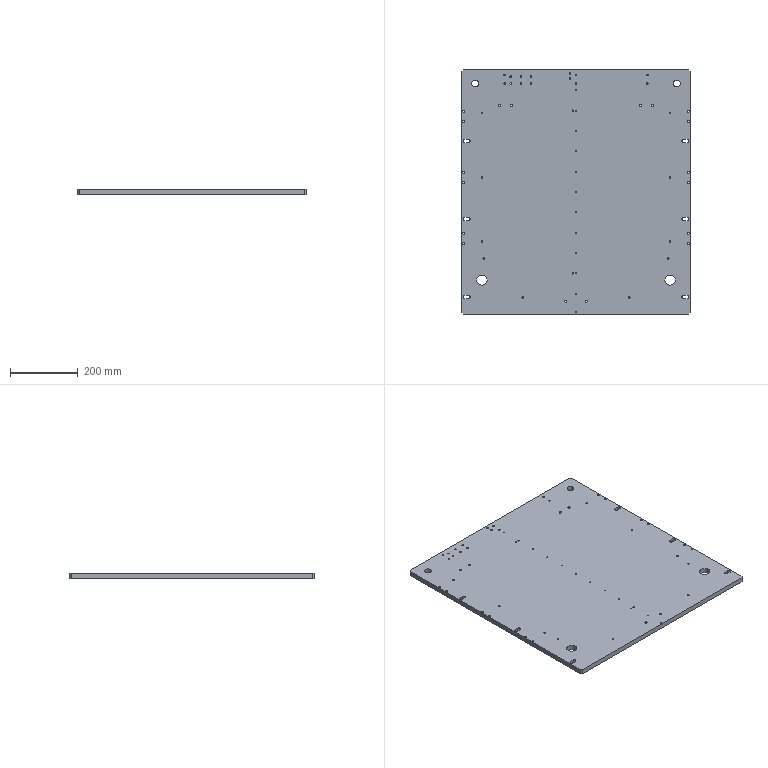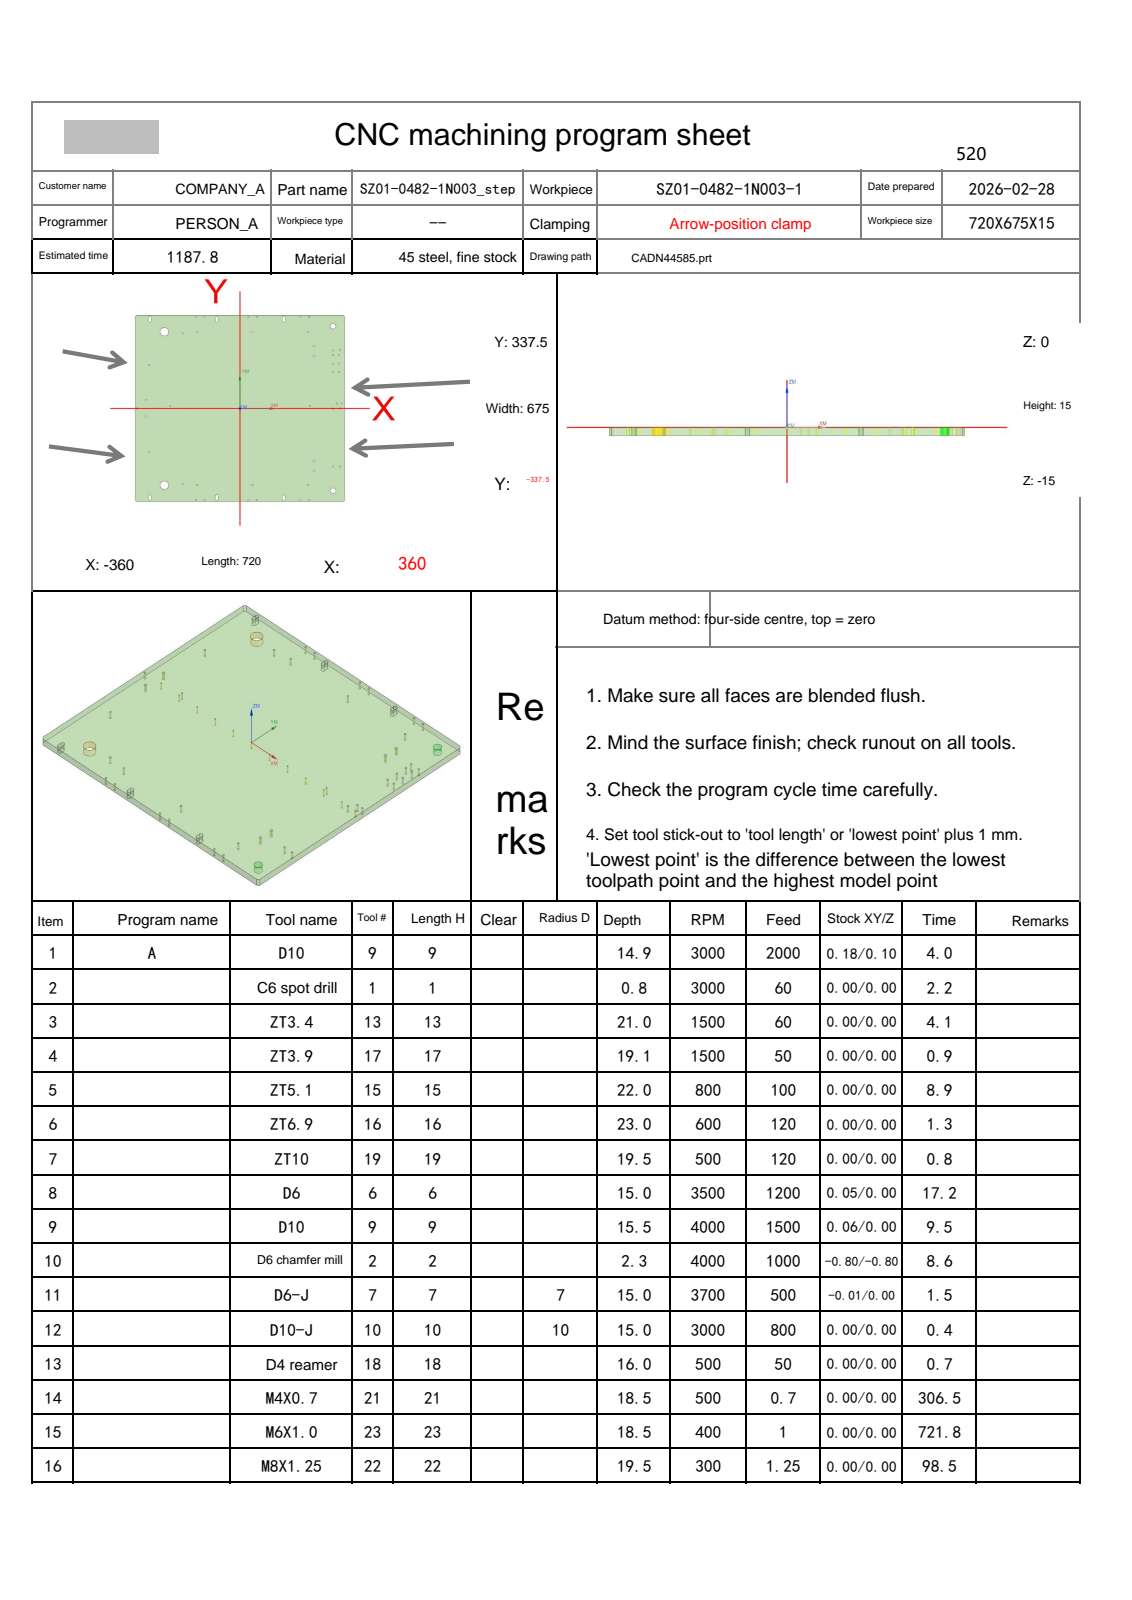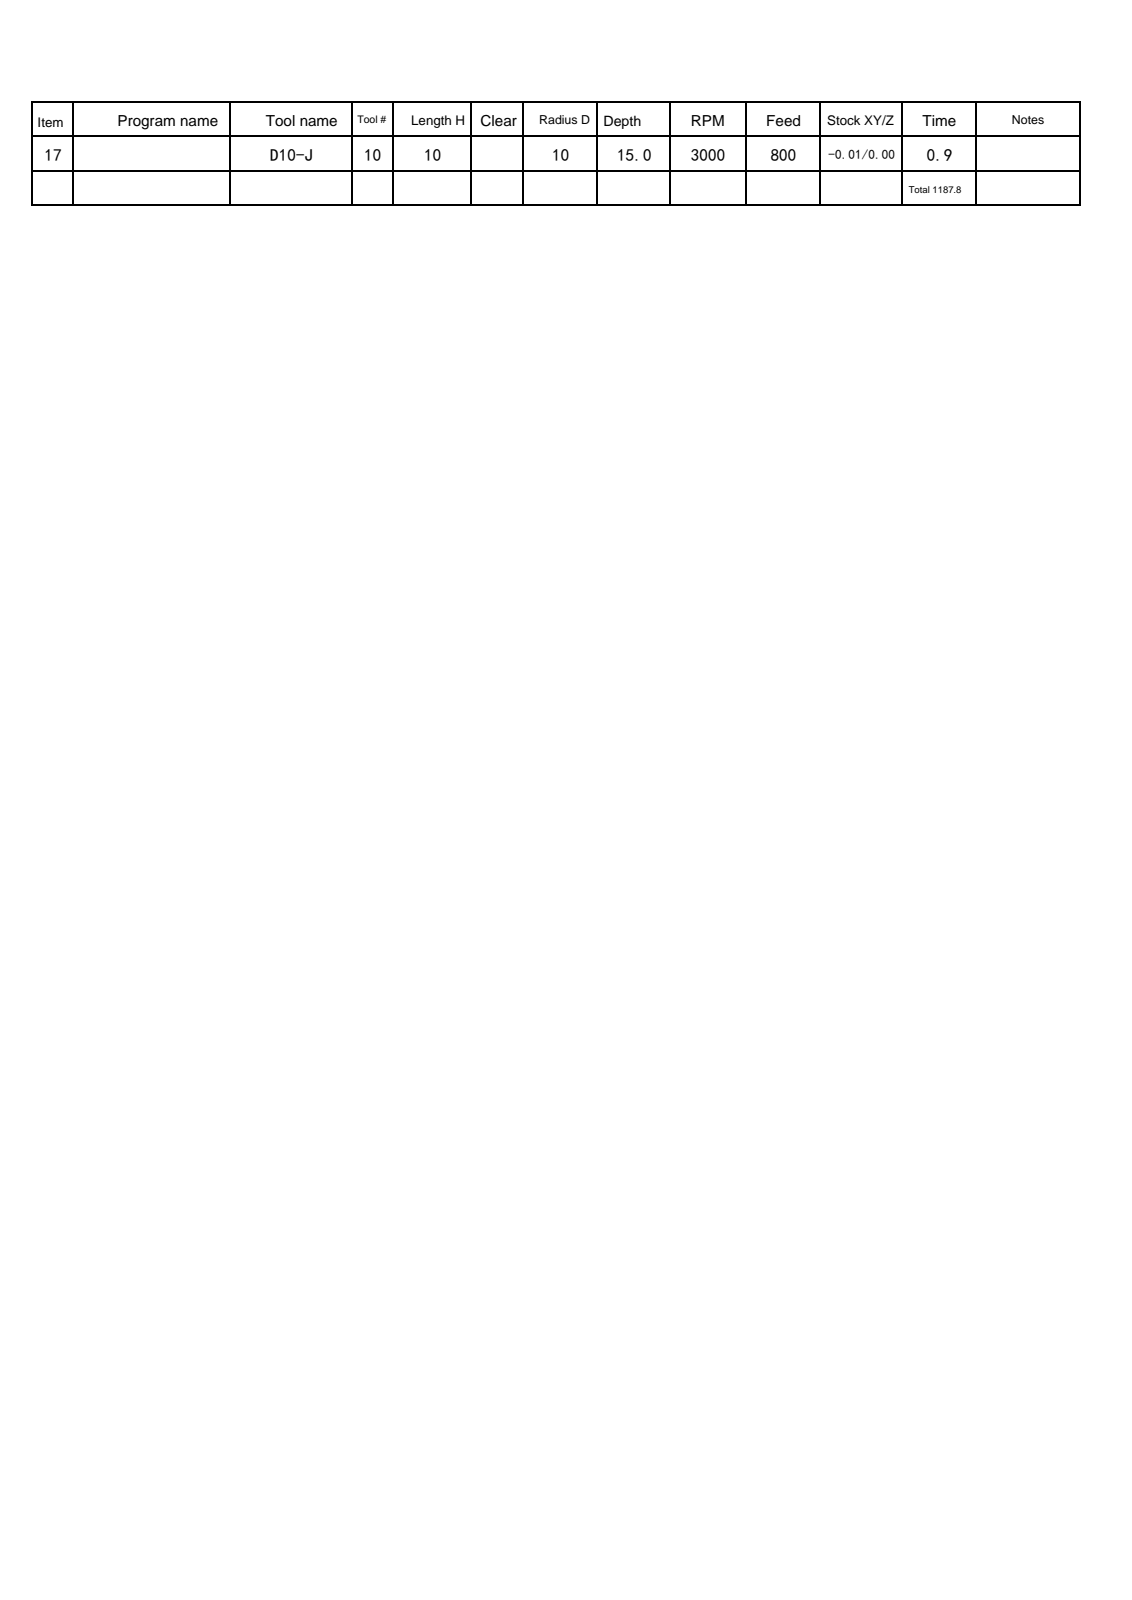NC program | NX | posted by the shop | part box 675 x 720 x 15 mm
Lines 5269 to 7670 of 7907, first 1495 of 2402 lines:
N9 T09 M06
(D10  D=10. R=0. H=09 ce=0.06 di=0.20)
G00 G90 G54 X320. Y-297.5 M03 S4000
G43 H09 Z60.
M08
Z.5
G03 X317.53 Y-299.97 I0.0 J-2.47 F1500.
X320. Y-302.44 I2.47 J0.0
X320. Y-302.44 Z.25 I0.0 J4.94
X320. Y-302.44 Z0.0 I0.0 J4.94
X320. Y-302.44 Z-.25 I0.0 J4.94
X320. Y-302.44 Z-.5 I0.0 J4.94
X320. Y-302.44 Z-.75 I0.0 J4.94
X320. Y-302.44 Z-1. I0.0 J4.94
X320. Y-302.44 Z-1.25 I0.0 J4.94
X320. Y-302.44 Z-1.5 I0.0 J4.94
X320. Y-302.44 Z-1.75 I0.0 J4.94
X320. Y-302.44 Z-2. I0.0 J4.94
X320. Y-302.44 Z-2.25 I0.0 J4.94
X320. Y-302.44 Z-2.5 I0.0 J4.94
X320. Y-302.44 Z-2.75 I0.0 J4.94
X320. Y-302.44 Z-3. I0.0 J4.94
X320. Y-302.44 Z-3.25 I0.0 J4.94
X320. Y-302.44 Z-3.5 I0.0 J4.94
X320. Y-302.44 Z-3.75 I0.0 J4.94
X320. Y-302.44 Z-4. I0.0 J4.94
X320. Y-302.44 Z-4.25 I0.0 J4.94
X320. Y-302.44 Z-4.5 I0.0 J4.94
X320. Y-302.44 Z-4.75 I0.0 J4.94
X320. Y-302.44 Z-5. I0.0 J4.94
X320. Y-302.44 Z-5.25 I0.0 J4.94
X320. Y-302.44 Z-5.5 I0.0 J4.94
X320. Y-302.44 Z-5.75 I0.0 J4.94
X320. Y-302.44 Z-6. I0.0 J4.94
X320. Y-302.44 Z-6.25 I0.0 J4.94
X320. Y-302.44 Z-6.5 I0.0 J4.94
X320. Y-302.44 Z-6.75 I0.0 J4.94
X320. Y-302.44 Z-7. I0.0 J4.94
X320. Y-302.44 Z-7.25 I0.0 J4.94
X320. Y-302.44 Z-7.5 I0.0 J4.94
X320. Y-302.44 Z-7.75 I0.0 J4.94
X320. Y-302.44 Z-8. I0.0 J4.94
X320. Y-302.44 Z-8.25 I0.0 J4.94
X320. Y-302.44 Z-8.5 I0.0 J4.94
X320. Y-302.44 Z-8.75 I0.0 J4.94
X320. Y-302.44 Z-9. I0.0 J4.94
X320. Y-302.44 Z-9.25 I0.0 J4.94
X320. Y-302.44 Z-9.5 I0.0 J4.94
X320. Y-302.44 Z-9.75 I0.0 J4.94
X320. Y-302.44 Z-10. I0.0 J4.94
X320. Y-302.44 Z-10.25 I0.0 J4.94
X320. Y-302.44 Z-10.5 I0.0 J4.94
X320. Y-302.44 Z-10.75 I0.0 J4.94
X320. Y-302.44 Z-11. I0.0 J4.94
X320. Y-302.44 Z-11.25 I0.0 J4.94
X320. Y-302.44 Z-11.5 I0.0 J4.94
X320. Y-302.44 Z-11.75 I0.0 J4.94
X320. Y-302.44 Z-12. I0.0 J4.94
X320. Y-302.44 Z-12.25 I0.0 J4.94
X320. Y-302.44 Z-12.5 I0.0 J4.94
X320. Y-302.44 Z-12.75 I0.0 J4.94
X320. Y-302.44 Z-13. I0.0 J4.94
X320. Y-302.44 Z-13.25 I0.0 J4.94
X320. Y-302.44 Z-13.5 I0.0 J4.94
X320. Y-302.44 Z-13.75 I0.0 J4.94
X320. Y-302.44 Z-14. I0.0 J4.94
X320. Y-302.44 Z-14.25 I0.0 J4.94
X320. Y-302.44 Z-14.5 I0.0 J4.94
X320. Y-302.44 Z-14.75 I0.0 J4.94
X320. Y-302.44 Z-15. I0.0 J4.94
X320. Y-302.44 Z-15.25 I0.0 J4.94
X320. Y-302.44 Z-15.5 I0.0 J4.94
X324.94 Y-297.5 I0.0 J4.94
X320. Y-292.56 I-4.94 J0.0
X315.06 Y-297.5 I0.0 J-4.94
X320. Y-302.44 I4.94 J0.0
X322.47 Y-299.97 I0.0 J2.47
X320. Y-297.5 I-2.47 J0.0
G00 Z60.
Y297.5
Z.5
G03 X317.53 Y295.03 I0.0 J-2.47
X320. Y292.56 I2.47 J0.0
X320. Y292.56 Z.25 I0.0 J4.94
X320. Y292.56 Z0.0 I0.0 J4.94
X320. Y292.56 Z-.25 I0.0 J4.94
X320. Y292.56 Z-.5 I0.0 J4.94
X320. Y292.56 Z-.75 I0.0 J4.94
X320. Y292.56 Z-1. I0.0 J4.94
X320. Y292.56 Z-1.25 I0.0 J4.94
X320. Y292.56 Z-1.5 I0.0 J4.94
X320. Y292.56 Z-1.75 I0.0 J4.94
X320. Y292.56 Z-2. I0.0 J4.94
X320. Y292.56 Z-2.25 I0.0 J4.94
X320. Y292.56 Z-2.5 I0.0 J4.94
X320. Y292.56 Z-2.75 I0.0 J4.94
X320. Y292.56 Z-3. I0.0 J4.94
X320. Y292.56 Z-3.25 I0.0 J4.94
X320. Y292.56 Z-3.5 I0.0 J4.94
X320. Y292.56 Z-3.75 I0.0 J4.94
X320. Y292.56 Z-4. I0.0 J4.94
X320. Y292.56 Z-4.25 I0.0 J4.94
X320. Y292.56 Z-4.5 I0.0 J4.94
X320. Y292.56 Z-4.75 I0.0 J4.94
X320. Y292.56 Z-5. I0.0 J4.94
X320. Y292.56 Z-5.25 I0.0 J4.94
X320. Y292.56 Z-5.5 I0.0 J4.94
X320. Y292.56 Z-5.75 I0.0 J4.94
X320. Y292.56 Z-6. I0.0 J4.94
X320. Y292.56 Z-6.25 I0.0 J4.94
X320. Y292.56 Z-6.5 I0.0 J4.94
X320. Y292.56 Z-6.75 I0.0 J4.94
X320. Y292.56 Z-7. I0.0 J4.94
X320. Y292.56 Z-7.25 I0.0 J4.94
X320. Y292.56 Z-7.5 I0.0 J4.94
X320. Y292.56 Z-7.75 I0.0 J4.94
X320. Y292.56 Z-8. I0.0 J4.94
X320. Y292.56 Z-8.25 I0.0 J4.94
X320. Y292.56 Z-8.5 I0.0 J4.94
X320. Y292.56 Z-8.75 I0.0 J4.94
X320. Y292.56 Z-9. I0.0 J4.94
X320. Y292.56 Z-9.25 I0.0 J4.94
X320. Y292.56 Z-9.5 I0.0 J4.94
X320. Y292.56 Z-9.75 I0.0 J4.94
X320. Y292.56 Z-10. I0.0 J4.94
X320. Y292.56 Z-10.25 I0.0 J4.94
X320. Y292.56 Z-10.5 I0.0 J4.94
X320. Y292.56 Z-10.75 I0.0 J4.94
X320. Y292.56 Z-11. I0.0 J4.94
X320. Y292.56 Z-11.25 I0.0 J4.94
X320. Y292.56 Z-11.5 I0.0 J4.94
X320. Y292.56 Z-11.75 I0.0 J4.94
X320. Y292.56 Z-12. I0.0 J4.94
X320. Y292.56 Z-12.25 I0.0 J4.94
X320. Y292.56 Z-12.5 I0.0 J4.94
X320. Y292.56 Z-12.75 I0.0 J4.94
X320. Y292.56 Z-13. I0.0 J4.94
X320. Y292.56 Z-13.25 I0.0 J4.94
X320. Y292.56 Z-13.5 I0.0 J4.94
X320. Y292.56 Z-13.75 I0.0 J4.94
X320. Y292.56 Z-14. I0.0 J4.94
X320. Y292.56 Z-14.25 I0.0 J4.94
X320. Y292.56 Z-14.5 I0.0 J4.94
X320. Y292.56 Z-14.75 I0.0 J4.94
X320. Y292.56 Z-15. I0.0 J4.94
X320. Y292.56 Z-15.25 I0.0 J4.94
X320. Y292.56 Z-15.5 I0.0 J4.94
X324.94 Y297.5 I0.0 J4.94
X320. Y302.44 I-4.94 J0.0
X315.06 Y297.5 I0.0 J-4.94
X320. Y292.56 I4.94 J0.0
X322.47 Y295.03 I0.0 J2.47
X320. Y297.5 I-2.47 J0.0
G00 Z60.
G00 G90 X-260. Y-277.5 M03 S4000
Z60.
Z.5
G03 X-264.97 Y-282.47 I0.0 J-4.97 F1500.
X-260. Y-287.44 I4.97 J0.0
X-260. Y-287.44 Z.3 I0.0 J9.94
X-260. Y-287.44 Z.1 I0.0 J9.94
X-260. Y-287.44 Z-.1 I0.0 J9.94
X-260. Y-287.44 Z-.3 I0.0 J9.94
X-260. Y-287.44 Z-.5 I0.0 J9.94
X-260. Y-287.44 Z-.7 I0.0 J9.94
X-260. Y-287.44 Z-.9 I0.0 J9.94
X-260. Y-287.44 Z-1.1 I0.0 J9.94
X-260. Y-287.44 Z-1.3 I0.0 J9.94
X-260. Y-287.44 Z-1.5 I0.0 J9.94
X-260. Y-287.44 Z-1.7 I0.0 J9.94
X-260. Y-287.44 Z-1.9 I0.0 J9.94
X-260. Y-287.44 Z-2.1 I0.0 J9.94
X-260. Y-287.44 Z-2.3 I0.0 J9.94
X-260. Y-287.44 Z-2.5 I0.0 J9.94
X-260. Y-287.44 Z-2.7 I0.0 J9.94
X-260. Y-287.44 Z-2.9 I0.0 J9.94
X-260. Y-287.44 Z-3.1 I0.0 J9.94
X-260. Y-287.44 Z-3.3 I0.0 J9.94
X-260. Y-287.44 Z-3.5 I0.0 J9.94
X-260. Y-287.44 Z-3.7 I0.0 J9.94
X-260. Y-287.44 Z-3.9 I0.0 J9.94
X-260. Y-287.44 Z-4.1 I0.0 J9.94
X-260. Y-287.44 Z-4.3 I0.0 J9.94
X-260. Y-287.44 Z-4.5 I0.0 J9.94
X-260. Y-287.44 Z-4.7 I0.0 J9.94
X-260. Y-287.44 Z-4.9 I0.0 J9.94
X-260. Y-287.44 Z-5.1 I0.0 J9.94
X-260. Y-287.44 Z-5.3 I0.0 J9.94
X-260. Y-287.44 Z-5.5 I0.0 J9.94
X-260. Y-287.44 Z-5.7 I0.0 J9.94
X-260. Y-287.44 Z-5.9 I0.0 J9.94
X-260. Y-287.44 Z-6.1 I0.0 J9.94
X-260. Y-287.44 Z-6.3 I0.0 J9.94
X-260. Y-287.44 Z-6.5 I0.0 J9.94
X-260. Y-287.44 Z-6.7 I0.0 J9.94
X-260. Y-287.44 Z-6.9 I0.0 J9.94
X-260. Y-287.44 Z-7.1 I0.0 J9.94
X-260. Y-287.44 Z-7.3 I0.0 J9.94
X-260. Y-287.44 Z-7.5 I0.0 J9.94
X-260. Y-287.44 Z-7.7 I0.0 J9.94
X-260. Y-287.44 Z-7.9 I0.0 J9.94
X-260. Y-287.44 Z-8.1 I0.0 J9.94
X-260. Y-287.44 Z-8.3 I0.0 J9.94
X-260. Y-287.44 Z-8.5 I0.0 J9.94
X-260. Y-287.44 Z-8.7 I0.0 J9.94
X-260. Y-287.44 Z-8.9 I0.0 J9.94
X-260. Y-287.44 Z-9.1 I0.0 J9.94
X-260. Y-287.44 Z-9.3 I0.0 J9.94
X-260. Y-287.44 Z-9.5 I0.0 J9.94
X-260. Y-287.44 Z-9.7 I0.0 J9.94
X-260. Y-287.44 Z-9.9 I0.0 J9.94
X-260. Y-287.44 Z-10.1 I0.0 J9.94
X-260. Y-287.44 Z-10.3 I0.0 J9.94
X-260. Y-287.44 Z-10.5 I0.0 J9.94
X-260. Y-287.44 Z-10.7 I0.0 J9.94
X-260. Y-287.44 Z-10.9 I0.0 J9.94
X-260. Y-287.44 Z-11.1 I0.0 J9.94
X-260. Y-287.44 Z-11.3 I0.0 J9.94
X-260. Y-287.44 Z-11.5 I0.0 J9.94
X-260. Y-287.44 Z-11.7 I0.0 J9.94
X-260. Y-287.44 Z-11.9 I0.0 J9.94
X-260. Y-287.44 Z-12.1 I0.0 J9.94
X-260. Y-287.44 Z-12.3 I0.0 J9.94
X-260. Y-287.44 Z-12.5 I0.0 J9.94
X-260. Y-287.44 Z-12.7 I0.0 J9.94
X-260. Y-287.44 Z-12.9 I0.0 J9.94
X-260. Y-287.44 Z-13.1 I0.0 J9.94
X-260. Y-287.44 Z-13.3 I0.0 J9.94
X-260. Y-287.44 Z-13.5 I0.0 J9.94
X-260. Y-287.44 Z-13.7 I0.0 J9.94
X-260. Y-287.44 Z-13.9 I0.0 J9.94
X-260. Y-287.44 Z-14.1 I0.0 J9.94
X-260. Y-287.44 Z-14.3 I0.0 J9.94
X-260. Y-287.44 Z-14.5 I0.0 J9.94
X-260. Y-287.44 Z-14.7 I0.0 J9.94
X-260. Y-287.44 Z-14.9 I0.0 J9.94
X-260. Y-267.56 Z-15. I0.0 J9.94
X-269.94 Y-277.5 I0.0 J-9.94
X-260. Y-287.44 I9.94 J0.0
X-250.06 Y-277.5 I0.0 J9.94
X-260. Y-267.56 I-9.94 J0.0
X-264.97 Y-272.53 I0.0 J-4.97
X-260. Y-277.5 I4.97 J0.0
G00 Z60.
Y277.5
Z.5
G03 X-264.97 Y272.53 I0.0 J-4.97
X-260. Y267.56 I4.97 J0.0
X-260. Y267.56 Z.3 I0.0 J9.94
X-260. Y267.56 Z.1 I0.0 J9.94
X-260. Y267.56 Z-.1 I0.0 J9.94
X-260. Y267.56 Z-.3 I0.0 J9.94
X-260. Y267.56 Z-.5 I0.0 J9.94
X-260. Y267.56 Z-.7 I0.0 J9.94
X-260. Y267.56 Z-.9 I0.0 J9.94
X-260. Y267.56 Z-1.1 I0.0 J9.94
X-260. Y267.56 Z-1.3 I0.0 J9.94
X-260. Y267.56 Z-1.5 I0.0 J9.94
X-260. Y267.56 Z-1.7 I0.0 J9.94
X-260. Y267.56 Z-1.9 I0.0 J9.94
X-260. Y267.56 Z-2.1 I0.0 J9.94
X-260. Y267.56 Z-2.3 I0.0 J9.94
X-260. Y267.56 Z-2.5 I0.0 J9.94
X-260. Y267.56 Z-2.7 I0.0 J9.94
X-260. Y267.56 Z-2.9 I0.0 J9.94
X-260. Y267.56 Z-3.1 I0.0 J9.94
X-260. Y267.56 Z-3.3 I0.0 J9.94
X-260. Y267.56 Z-3.5 I0.0 J9.94
X-260. Y267.56 Z-3.7 I0.0 J9.94
X-260. Y267.56 Z-3.9 I0.0 J9.94
X-260. Y267.56 Z-4.1 I0.0 J9.94
X-260. Y267.56 Z-4.3 I0.0 J9.94
X-260. Y267.56 Z-4.5 I0.0 J9.94
X-260. Y267.56 Z-4.7 I0.0 J9.94
X-260. Y267.56 Z-4.9 I0.0 J9.94
X-260. Y267.56 Z-5.1 I0.0 J9.94
X-260. Y267.56 Z-5.3 I0.0 J9.94
X-260. Y267.56 Z-5.5 I0.0 J9.94
X-260. Y267.56 Z-5.7 I0.0 J9.94
X-260. Y267.56 Z-5.9 I0.0 J9.94
X-260. Y267.56 Z-6.1 I0.0 J9.94
X-260. Y267.56 Z-6.3 I0.0 J9.94
X-260. Y267.56 Z-6.5 I0.0 J9.94
X-260. Y267.56 Z-6.7 I0.0 J9.94
X-260. Y267.56 Z-6.9 I0.0 J9.94
X-260. Y267.56 Z-7.1 I0.0 J9.94
X-260. Y267.56 Z-7.3 I0.0 J9.94
X-260. Y267.56 Z-7.5 I0.0 J9.94
X-260. Y267.56 Z-7.7 I0.0 J9.94
X-260. Y267.56 Z-7.9 I0.0 J9.94
X-260. Y267.56 Z-8.1 I0.0 J9.94
X-260. Y267.56 Z-8.3 I0.0 J9.94
X-260. Y267.56 Z-8.5 I0.0 J9.94
X-260. Y267.56 Z-8.7 I0.0 J9.94
X-260. Y267.56 Z-8.9 I0.0 J9.94
X-260. Y267.56 Z-9.1 I0.0 J9.94
X-260. Y267.56 Z-9.3 I0.0 J9.94
X-260. Y267.56 Z-9.5 I0.0 J9.94
X-260. Y267.56 Z-9.7 I0.0 J9.94
X-260. Y267.56 Z-9.9 I0.0 J9.94
X-260. Y267.56 Z-10.1 I0.0 J9.94
X-260. Y267.56 Z-10.3 I0.0 J9.94
X-260. Y267.56 Z-10.5 I0.0 J9.94
X-260. Y267.56 Z-10.7 I0.0 J9.94
X-260. Y267.56 Z-10.9 I0.0 J9.94
X-260. Y267.56 Z-11.1 I0.0 J9.94
X-260. Y267.56 Z-11.3 I0.0 J9.94
X-260. Y267.56 Z-11.5 I0.0 J9.94
X-260. Y267.56 Z-11.7 I0.0 J9.94
X-260. Y267.56 Z-11.9 I0.0 J9.94
X-260. Y267.56 Z-12.1 I0.0 J9.94
X-260. Y267.56 Z-12.3 I0.0 J9.94
X-260. Y267.56 Z-12.5 I0.0 J9.94
X-260. Y267.56 Z-12.7 I0.0 J9.94
X-260. Y267.56 Z-12.9 I0.0 J9.94
X-260. Y267.56 Z-13.1 I0.0 J9.94
X-260. Y267.56 Z-13.3 I0.0 J9.94
X-260. Y267.56 Z-13.5 I0.0 J9.94
X-260. Y267.56 Z-13.7 I0.0 J9.94
X-260. Y267.56 Z-13.9 I0.0 J9.94
X-260. Y267.56 Z-14.1 I0.0 J9.94
X-260. Y267.56 Z-14.3 I0.0 J9.94
X-260. Y267.56 Z-14.5 I0.0 J9.94
X-260. Y267.56 Z-14.7 I0.0 J9.94
X-260. Y267.56 Z-14.9 I0.0 J9.94
X-260. Y287.44 Z-15. I0.0 J9.94
X-269.94 Y277.5 I0.0 J-9.94
X-260. Y267.56 I9.94 J0.0
X-250.06 Y277.5 I0.0 J9.94
X-260. Y287.44 I-9.94 J0.0
X-264.97 Y282.47 I0.0 J-4.97
X-260. Y277.5 I4.97 J0.0
G00 Z60.
G91 G28 Z0.0
M05
M09
G91 G28 Z0.0
M01
N10 T02 M06
(D6 chamfer mill  D=6. R=0. H=02 ce=0.00 di=0.00)
G00 G90 G54 X-300. Y0.0 M03 S4000
G43 H02 Z30.
M08
G98 G81 X-300. Y0.0 Z-2.2 R3. F80.
X-240.
X-180.
X-120.
X-60.
X0.0
X60.
X120.
X180.
X240.
X300.
G80
G00 Z30.
G00 G90 X240. Y9.5 M03 S4000
Z30.
G98 G81 X240. Y9.5 Z-2.3 R3. F80.
X-240.
G80
G00 Z30.
G00 G90 X321.021 Y.409 M03 S4000
Z60.
Z-.6
G01 Z-1.1 F300.
X321.5 Y.6
G03 X320. Y2.1 I-1.5 J0.0
X317.9 Y0.0 I0.0 J-2.1
X320. Y-2.1 I2.1 J0.0
X322.1 Y0.0 I0.0 J2.1
X320. Y2.1 I-2.1 J0.0
X318.5 Y.6 I0.0 J-1.5
G01 X318.979 Y.409
Z-.6
G00 Z60.
X346.021
Z-.6
G01 Z-1.1
X346.5 Y.6
G03 X345. Y2.1 I-1.5 J0.0
X342.9 Y0.0 I0.0 J-2.1
X345. Y-2.1 I2.1 J0.0
X347.1 Y0.0 I0.0 J2.1
X345. Y2.1 I-2.1 J0.0
X343.5 Y.6 I0.0 J-1.5
G01 X343.979 Y.409
Z-.6
G00 Z60.
X351.021 Y18.409
Z-.6
G01 Z-1.1
X351.5 Y18.6
G03 X350. Y20.1 I-1.5 J0.0
X347.9 Y18. I0.0 J-2.1
X350. Y15.9 I2.1 J0.0
X352.1 Y18. I0.0 J2.1
X350. Y20.1 I-2.1 J0.0
X348.5 Y18.6 I0.0 J-1.5
G01 X348.979 Y18.409
Z-.6
G00 Z60.
X335.021
Z-.6
G01 Z-1.1
X335.5 Y18.6
G03 X334. Y20.1 I-1.5 J0.0
X331.9 Y18. I0.0 J-2.1
X334. Y15.9 I2.1 J0.0
X336.1 Y18. I0.0 J2.1
X334. Y20.1 I-2.1 J0.0
X332.5 Y18.6 I0.0 J-1.5
G01 X332.979 Y18.409
Z-.6
G00 Z60.
X318.979 Y132.091
Z-.6
G01 Z-1.1
X318.5 Y131.9
G03 X320. Y130.4 I1.5 J0.0
X322.1 Y132.5 I0.0 J2.1
X320. Y134.6 I-2.1 J0.0
X317.9 Y132.5 I0.0 J-2.1
X320. Y130.4 I2.1 J0.0
X321.5 Y131.9 I0.0 J1.5
G01 X321.021 Y132.091
Z-.6
G00 Z60.
X338.979
Z-.6
G01 Z-1.1
X338.5 Y131.9
G03 X340. Y130.4 I1.5 J0.0
X342.1 Y132.5 I0.0 J2.1
X340. Y134.6 I-2.1 J0.0
X337.9 Y132.5 I0.0 J-2.1
X340. Y130.4 I2.1 J0.0
X341.5 Y131.9 I0.0 J1.5
G01 X341.021 Y132.091
Z-.6
G00 Z60.
X338.979 Y162.091
Z-.6
G01 Z-1.1
X338.5 Y161.9
G03 X340. Y160.4 I1.5 J0.0
X342.1 Y162.5 I0.0 J2.1
X340. Y164.6 I-2.1 J0.0
X337.9 Y162.5 I0.0 J-2.1
X340. Y160.4 I2.1 J0.0
X341.5 Y161.9 I0.0 J1.5
G01 X341.021 Y162.091
Z-.6
G00 Z60.
X318.979
Z-.6
G01 Z-1.1
X318.5 Y161.9
G03 X320. Y160.4 I1.5 J0.0
X322.1 Y162.5 I0.0 J2.1
X320. Y164.6 I-2.1 J0.0
X317.9 Y162.5 I0.0 J-2.1
X320. Y160.4 I2.1 J0.0
X321.5 Y161.9 I0.0 J1.5
G01 X321.021 Y162.091
Z-.6
G00 Z60.
X318.979 Y192.091
Z-.6
G01 Z-1.1
X318.5 Y191.9
G03 X320. Y190.4 I1.5 J0.0
X322.1 Y192.5 I0.0 J2.1
X320. Y194.6 I-2.1 J0.0
X317.9 Y192.5 I0.0 J-2.1
X320. Y190.4 I2.1 J0.0
X321.5 Y191.9 I0.0 J1.5
G01 X321.021 Y192.091
Z-.6
G00 Z60.
X338.979
Z-.6
G01 Z-1.1
X338.5 Y191.9
G03 X340. Y190.4 I1.5 J0.0
X342.1 Y192.5 I0.0 J2.1
X340. Y194.6 I-2.1 J0.0
X337.9 Y192.5 I0.0 J-2.1
X340. Y190.4 I2.1 J0.0
X341.5 Y191.9 I0.0 J1.5
G01 X341.021 Y192.091
Z-.6
G00 Z60.
X346.021 Y210.409
Z-.6
G01 Z-1.1
X346.5 Y210.6
G03 X345. Y212.1 I-1.5 J0.0
X342.9 Y210. I0.0 J-2.1
X345. Y207.9 I2.1 J0.0
X347.1 Y210. I0.0 J2.1
X345. Y212.1 I-2.1 J0.0
X343.5 Y210.6 I0.0 J-1.5
G01 X343.979 Y210.409
Z-.6
G00 Z60.
X321.021
Z-.6
G01 Z-1.1
X321.5 Y210.6
G03 X320. Y212.1 I-1.5 J0.0
X317.9 Y210. I0.0 J-2.1
X320. Y207.9 I2.1 J0.0
X322.1 Y210. I0.0 J2.1
X320. Y212.1 I-2.1 J0.0
X318.5 Y210.6 I0.0 J-1.5
G01 X318.979 Y210.409
Z-.6
G00 Z60.
X234.021 Y277.409
Z-.6
G01 Z-1.1
X234.5 Y277.6
G03 X233. Y279.1 I-1.5 J0.0
X230.9 Y277. I0.0 J-2.1
X233. Y274.9 I2.1 J0.0
X235.1 Y277. I0.0 J2.1
X233. Y279.1 I-2.1 J0.0
X231.5 Y277.6 I0.0 J-1.5
G01 X231.979 Y277.409
Z-.6
G00 Z60.
X239.021 Y331.909
Z-.6
G01 Z-1.1
X239.5 Y332.1
G03 X238. Y333.6 I-1.5 J0.0
X235.9 Y331.5 I0.0 J-2.1
X238. Y329.4 I2.1 J0.0
X240.1 Y331.5 I0.0 J2.1
X238. Y333.6 I-2.1 J0.0
X236.5 Y332.1 I0.0 J-1.5
G01 X236.979 Y331.909
Z-.6
G00 Z60.
X209.021
Z-.6
G01 Z-1.1
X209.5 Y332.1
G03 X208. Y333.6 I-1.5 J0.0
X205.9 Y331.5 I0.0 J-2.1
X208. Y329.4 I2.1 J0.0
X210.1 Y331.5 I0.0 J2.1
X208. Y333.6 I-2.1 J0.0
X206.5 Y332.1 I0.0 J-1.5
G01 X206.979 Y331.909
Z-.6
G00 Z60.
X59.021
Z-.6
G01 Z-1.1
X59.5 Y332.1
G03 X58. Y333.6 I-1.5 J0.0
X55.9 Y331.5 I0.0 J-2.1
X58. Y329.4 I2.1 J0.0
X60.1 Y331.5 I0.0 J2.1
X58. Y333.6 I-2.1 J0.0
X56.5 Y332.1 I0.0 J-1.5
G01 X56.979 Y331.909
Z-.6
G00 Z60.
X44.021 Y277.409
Z-.6
G01 Z-1.1
X44.5 Y277.6
G03 X43. Y279.1 I-1.5 J0.0
X40.9 Y277. I0.0 J-2.1
X43. Y274.9 I2.1 J0.0
X45.1 Y277. I0.0 J2.1
X43. Y279.1 I-2.1 J0.0
X41.5 Y277.6 I0.0 J-1.5
G01 X41.979 Y277.409
Z-.6
G00 Z60.
X29.021 Y331.909
Z-.6
G01 Z-1.1
X29.5 Y332.1
G03 X28. Y333.6 I-1.5 J0.0
X25.9 Y331.5 I0.0 J-2.1
X28. Y329.4 I2.1 J0.0
X30.1 Y331.5 I0.0 J2.1
X28. Y333.6 I-2.1 J0.0
X26.5 Y332.1 I0.0 J-1.5
G01 X26.979 Y331.909
Z-.6
G00 Z60.
X-120.979
Z-.6
G01 Z-1.1
X-120.5 Y332.1
G03 X-122. Y333.6 I-1.5 J0.0
X-124.1 Y331.5 I0.0 J-2.1
X-122. Y329.4 I2.1 J0.0
X-119.9 Y331.5 I0.0 J2.1
X-122. Y333.6 I-2.1 J0.0
X-123.5 Y332.1 I0.0 J-1.5
G01 X-123.021 Y331.909
Z-.6
G00 Z60.
X-150.979
Z-.6
G01 Z-1.1
X-150.5 Y332.1
G03 X-152. Y333.6 I-1.5 J0.0
X-154.1 Y331.5 I0.0 J-2.1
X-152. Y329.4 I2.1 J0.0
X-149.9 Y331.5 I0.0 J2.1
X-152. Y333.6 I-2.1 J0.0
X-153.5 Y332.1 I0.0 J-1.5
G01 X-153.021 Y331.909
Z-.6
G00 Z60.
X-145.979 Y277.409
Z-.6
G01 Z-1.1
X-145.5 Y277.6
G03 X-147. Y279.1 I-1.5 J0.0
X-149.1 Y277. I0.0 J-2.1
X-147. Y274.9 I2.1 J0.0
X-144.9 Y277. I0.0 J2.1
X-147. Y279.1 I-2.1 J0.0
X-148.5 Y277.6 I0.0 J-1.5
G01 X-148.021 Y277.409
Z-.6
G00 Z60.
X-195.979 Y272.341
Z-.6
G01 Z-1.1
X-195.5 Y272.532
G03 X-197. Y274.032 I-1.5 J0.0
X-199.1 Y271.932 I0.0 J-2.1
X-197. Y269.832 I2.1 J0.0
X-194.9 Y271.932 I0.0 J2.1
X-197. Y274.032 I-2.1 J0.0
X-198.5 Y272.532 I0.0 J-1.5
G01 X-198.021 Y272.341
Z-.6
G00 Z60.
X-310.911 Y157.409
Z-.6
G01 Z-1.1
X-310.432 Y157.6
G03 X-311.932 Y159.1 I-1.5 J0.0
X-314.032 Y157. I0.0 J-2.1
X-311.932 Y154.9 I2.1 J0.0
X-309.832 Y157. I0.0 J2.1
X-311.932 Y159.1 I-2.1 J0.0
X-313.432 Y157.6 I0.0 J-1.5
G01 X-312.953 Y157.409
Z-.6
G00 Z60.
X-352.979 Y.409
Z-.6
G01 Z-1.1
X-352.5 Y.6
G03 X-354. Y2.1 I-1.5 J0.0
X-356.1 Y0.0 I0.0 J-2.1
X-354. Y-2.1 I2.1 J0.0
X-351.9 Y0.0 I0.0 J2.1
X-354. Y2.1 I-2.1 J0.0
X-355.5 Y.6 I0.0 J-1.5
G01 X-355.021 Y.409
Z-.6
G00 Z60.
X-310.911 Y-156.591
Z-.6
G01 Z-1.1
X-310.432 Y-156.4
G03 X-311.932 Y-154.9 I-1.5 J0.0
X-314.032 Y-157. I0.0 J-2.1
X-311.932 Y-159.1 I2.1 J0.0
X-309.832 Y-157. I0.0 J2.1
X-311.932 Y-154.9 I-2.1 J0.0
X-313.432 Y-156.4 I0.0 J-1.5
G01 X-312.953 Y-156.591
Z-.6
G00 Z60.
X-195.979 Y-271.523
Z-.6
G01 Z-1.1
X-195.5 Y-271.332
G03 X-197. Y-269.832 I-1.5 J0.0
X-199.1 Y-271.932 I0.0 J-2.1
X-197. Y-274.032 I2.1 J0.0
X-194.9 Y-271.932 I0.0 J2.1
X-197. Y-269.832 I-2.1 J0.0
X-198.5 Y-271.332 I0.0 J-1.5
G01 X-198.021 Y-271.523
Z-.6
G00 Z60.
X-145.979 Y-276.591
Z-.6
G01 Z-1.1
X-145.5 Y-276.4
G03 X-147. Y-274.9 I-1.5 J0.0
X-149.1 Y-277. I0.0 J-2.1
X-147. Y-279.1 I2.1 J0.0
X-144.9 Y-277. I0.0 J2.1
X-147. Y-274.9 I-2.1 J0.0
X-148.5 Y-276.4 I0.0 J-1.5
G01 X-148.021 Y-276.591
Z-.6
G00 Z60.
X-150.979 Y-331.091
Z-.6
G01 Z-1.1
X-150.5 Y-330.9
G03 X-152. Y-329.4 I-1.5 J0.0
X-154.1 Y-331.5 I0.0 J-2.1
X-152. Y-333.6 I2.1 J0.0
X-149.9 Y-331.5 I0.0 J2.1
X-152. Y-329.4 I-2.1 J0.0
X-153.5 Y-330.9 I0.0 J-1.5
G01 X-153.021 Y-331.091
Z-.6
G00 Z60.
X-120.979
Z-.6
G01 Z-1.1
X-120.5 Y-330.9
G03 X-122. Y-329.4 I-1.5 J0.0
X-124.1 Y-331.5 I0.0 J-2.1
X-122. Y-333.6 I2.1 J0.0
X-119.9 Y-331.5 I0.0 J2.1
X-122. Y-329.4 I-2.1 J0.0
X-123.5 Y-330.9 I0.0 J-1.5
G01 X-123.021 Y-331.091
Z-.6
G00 Z60.
X29.021
Z-.6
G01 Z-1.1
X29.5 Y-330.9
G03 X28. Y-329.4 I-1.5 J0.0
X25.9 Y-331.5 I0.0 J-2.1
X28. Y-333.6 I2.1 J0.0
X30.1 Y-331.5 I0.0 J2.1
X28. Y-329.4 I-2.1 J0.0
X26.5 Y-330.9 I0.0 J-1.5
G01 X26.979 Y-331.091
Z-.6
G00 Z60.
X44.021 Y-276.591
Z-.6
G01 Z-1.1
X44.5 Y-276.4
G03 X43. Y-274.9 I-1.5 J0.0
X40.9 Y-277. I0.0 J-2.1
X43. Y-279.1 I2.1 J0.0
X45.1 Y-277. I0.0 J2.1
X43. Y-274.9 I-2.1 J0.0
X41.5 Y-276.4 I0.0 J-1.5
G01 X41.979 Y-276.591
Z-.6
G00 Z60.
X59.021 Y-331.091
Z-.6
G01 Z-1.1
X59.5 Y-330.9
G03 X58. Y-329.4 I-1.5 J0.0
X55.9 Y-331.5 I0.0 J-2.1
X58. Y-333.6 I2.1 J0.0
X60.1 Y-331.5 I0.0 J2.1
X58. Y-329.4 I-2.1 J0.0
X56.5 Y-330.9 I0.0 J-1.5
G01 X56.979 Y-331.091
Z-.6
G00 Z60.
X209.021
Z-.6
G01 Z-1.1
X209.5 Y-330.9
G03 X208. Y-329.4 I-1.5 J0.0
X205.9 Y-331.5 I0.0 J-2.1
X208. Y-333.6 I2.1 J0.0
X210.1 Y-331.5 I0.0 J2.1
X208. Y-329.4 I-2.1 J0.0
X206.5 Y-330.9 I0.0 J-1.5
G01 X206.979 Y-331.091
Z-.6
G00 Z60.
X239.021
Z-.6
G01 Z-1.1
X239.5 Y-330.9
G03 X238. Y-329.4 I-1.5 J0.0
X235.9 Y-331.5 I0.0 J-2.1
X238. Y-333.6 I2.1 J0.0
X240.1 Y-331.5 I0.0 J2.1
X238. Y-329.4 I-2.1 J0.0
X236.5 Y-330.9 I0.0 J-1.5
G01 X236.979 Y-331.091
Z-.6
G00 Z60.
X234.021 Y-276.591
Z-.6
G01 Z-1.1
X234.5 Y-276.4
G03 X233. Y-274.9 I-1.5 J0.0
X230.9 Y-277. I0.0 J-2.1
X233. Y-279.1 I2.1 J0.0
X235.1 Y-277. I0.0 J2.1
X233. Y-274.9 I-2.1 J0.0
X231.5 Y-276.4 I0.0 J-1.5
G01 X231.979 Y-276.591
Z-.6
G00 Z60.
X321.021 Y-209.591
Z-.6
G01 Z-1.1
X321.5 Y-209.4
G03 X320. Y-207.9 I-1.5 J0.0
X317.9 Y-210. I0.0 J-2.1
X320. Y-212.1 I2.1 J0.0
X322.1 Y-210. I0.0 J2.1
X320. Y-207.9 I-2.1 J0.0
X318.5 Y-209.4 I0.0 J-1.5
G01 X318.979 Y-209.591
Z-.6
G00 Z60.
X346.021
Z-.6
G01 Z-1.1
X346.5 Y-209.4
G03 X345. Y-207.9 I-1.5 J0.0
X342.9 Y-210. I0.0 J-2.1
X345. Y-212.1 I2.1 J0.0
X347.1 Y-210. I0.0 J2.1
X345. Y-207.9 I-2.1 J0.0
X343.5 Y-209.4 I0.0 J-1.5
G01 X343.979 Y-209.591
Z-.6
G00 Z60.
G00 G90 X-320.5 Y30.8 M03 S4000
Z60.
Z-1.
G01 Z-1.5 F500.
Y31.2
G03 X-322. Y32.7 I-1.5 J0.0
X-324.7 Y30. I0.0 J-2.7
X-322. Y27.3 I2.7 J0.0
X-319.3 Y30. I0.0 J2.7
X-322. Y32.7 I-2.7 J0.0
X-323.5 Y31.2 I0.0 J-1.5
G01 Y30.8
Z-1.
G00 Z60.
X-320.5 Y-29.2
Z-1.
G01 Z-1.5
Y-28.8
G03 X-322. Y-27.3 I-1.5 J0.0
X-324.7 Y-30. I0.0 J-2.7
X-322. Y-32.7 I2.7 J0.0
X-319.3 Y-30. I0.0 J2.7
X-322. Y-27.3 I-2.7 J0.0
X-323.5 Y-28.8 I0.0 J-1.5
G01 Y-29.2
Z-1.
G00 Z60.
X256.5 Y-224.7
Z-1.
G01 Z-1.5
Y-224.3
G03 X255. Y-222.8 I-1.5 J0.0
X252.3 Y-225.5 I0.0 J-2.7
X255. Y-228.2 I2.7 J0.0
X257.7 Y-225.5 I0.0 J2.7
X255. Y-222.8 I-2.7 J0.0
X253.5 Y-224.3 I0.0 J-1.5
G01 Y-224.7
Z-1.
G00 Z60.
X256.5 Y-188.7
Z-1.
G01 Z-1.5
Y-188.3
G03 X255. Y-186.8 I-1.5 J0.0
X252.3 Y-189.5 I0.0 J-2.7
X255. Y-192.2 I2.7 J0.0
X257.7 Y-189.5 I0.0 J2.7
X255. Y-186.8 I-2.7 J0.0
X253.5 Y-188.3 I0.0 J-1.5
G01 Y-188.7
Z-1.
G00 Z60.
X256.5 Y190.3
Z-1.
G01 Z-1.5
Y190.7
G03 X255. Y192.2 I-1.5 J0.0
X252.3 Y189.5 I0.0 J-2.7
X255. Y186.8 I2.7 J0.0
X257.7 Y189.5 I0.0 J2.7
X255. Y192.2 I-2.7 J0.0
X253.5 Y190.7 I0.0 J-1.5
G01 Y190.3
Z-1.
G00 Z60.
X256.5 Y226.3
Z-1.
G01 Z-1.5
Y226.7
G03 X255. Y228.2 I-1.5 J0.0
X252.3 Y225.5 I0.0 J-2.7
X255. Y222.8 I2.7 J0.0
X257.7 Y225.5 I0.0 J2.7
X255. Y228.2 I-2.7 J0.0
X253.5 Y226.7 I0.0 J-1.5
G01 Y226.3
Z-1.
G00 Z60.
G00 G90 X-361.375 Y332.257 M03 S3500
Z60.
Z.055
G01 Z-1.2 F1000.
G03 X-361.069 Y332.423 I-.795 J1.835
G01 X-361.022 Y332.45
X-361. Y332.5
X-360.966 Y332.759
X-360.866 Y333.
X-360.707 Y333.207
X-355.707 Y338.207
X-355.5 Y338.366
X-355.259 Y338.466
X-355. Y338.5
X355.
X355.259 Y338.466
X355.5 Y338.366
X355.707 Y338.207
X360.707 Y333.207
X360.744 Y333.167
X360.797 Y333.155
G03 X361.14 Y333.095 I.518 J1.932
G01 Z.113
G00 Z60.
Y-333.095
Z.113
G01 Z-1.2
G03 X360.797 Y-333.155 I.174 J-1.992
G01 X360.744 Y-333.167
X360.707 Y-333.207
X355.707 Y-338.207
X355.5 Y-338.366
X355.259 Y-338.466
X355. Y-338.5
X-355.
X-355.259 Y-338.466
X-355.5 Y-338.366
X-355.707 Y-338.207
X-360.707 Y-333.207
X-360.744 Y-333.167
X-360.797 Y-333.155
G03 X-361.14 Y-333.095 I-.518 J-1.932
G01 Z.113
G00 Z60.
X-313.773 Y-322.114
Z.172
G01 Z-1.2
G03 X-313.973 Y-322.4 I1.532 J-1.286
G01 X-314.003 Y-322.446
X-314. Y-322.5
Y-327.5
G03 X-310. Y-331.5 I4. J0.0
X-306. Y-327.5 I0.0 J4.
G01 Y-317.5
G03 X-310. Y-313.5 I-4. J0.0
X-314. Y-317.5 I0.0 J-4.
G01 Y-322.5
X-314.003 Y-322.554
X-313.973 Y-322.6
G03 X-313.773 Y-322.886 I1.732 J1.
G01 Z.172
G00 Z60.
X-311.525 Y-155.685
Z.284
G01 Z-1.2
G03 X-311.83 Y-155.516 I-1.118 J-1.658
G01 X-311.878 Y-155.491
X-311.932 Y-155.5
G03 X-313.432 Y-157. I0.0 J-1.5
X-311.932 Y-158.5 I1.5 J0.0
X-310.432 Y-157. I0.0 J1.5
X-311.932 Y-155.5 I-1.5 J0.0
G01 X-311.986 Y-155.491
X-312.034 Y-155.516
G03 X-312.339 Y-155.685 I.813 J-1.827
G01 Z.284
G00 Z60.
X-259.606 Y-263.712
Z.196
G01 Z-1.2
G03 X-259.899 Y-263.523 I-1.227 J-1.579
G01 X-259.946 Y-263.495
X-260. Y-263.5
G03 X-274. Y-277.5 I0.0 J-14.
X-260. Y-291.5 I14. J0.0
X-246. Y-277.5 I0.0 J14.
X-260. Y-263.5 I-14. J0.0
G01 X-260.054 Y-263.495
X-260.101 Y-263.523
G03 X-260.394 Y-263.712 I.935 J-1.768
G01 Z.196
G00 Z60.
X-196.593 Y-270.617
Z.284
G01 Z-1.2
G03 X-196.898 Y-270.448 I-1.118 J-1.658
G01 X-196.946 Y-270.423
X-197. Y-270.432
G03 X-198.5 Y-271.932 I0.0 J-1.5
X-197. Y-273.432 I1.5 J0.0
X-195.5 Y-271.932 I0.0 J1.5
X-197. Y-270.432 I-1.5 J0.0
G01 X-197.054 Y-270.423
X-197.102 Y-270.448
G03 X-197.407 Y-270.617 I.813 J-1.827
G01 Z.284
G00 Z60.
X-146.593 Y-275.685
Z.284
G01 Z-1.2
G03 X-146.898 Y-275.516 I-1.118 J-1.658
G01 X-146.946 Y-275.491
X-147. Y-275.5
G03 X-148.5 Y-277. I0.0 J-1.5
X-147. Y-278.5 I1.5 J0.0
X-145.5 Y-277. I0.0 J1.5
X-147. Y-275.5 I-1.5 J0.0
G01 X-147.054 Y-275.491
X-147.102 Y-275.516
G03 X-147.407 Y-275.685 I.813 J-1.827
G01 Z.284
G00 Z60.
X-151.593 Y-330.185
Z.284
G01 Z-1.2
G03 X-151.898 Y-330.016 I-1.118 J-1.658
G01 X-151.946 Y-329.991
X-152. Y-330.
G03 X-153.5 Y-331.5 I0.0 J-1.5
X-152. Y-333. I1.5 J0.0
X-150.5 Y-331.5 I0.0 J1.5
X-152. Y-330. I-1.5 J0.0
G01 X-152.054 Y-329.991
X-152.102 Y-330.016
G03 X-152.407 Y-330.185 I.813 J-1.827
G01 Z.284
G00 Z60.
X-121.593
Z.284
G01 Z-1.2
G03 X-121.898 Y-330.016 I-1.118 J-1.658
G01 X-121.946 Y-329.991
X-122. Y-330.
G03 X-123.5 Y-331.5 I0.0 J-1.5
X-122. Y-333. I1.5 J0.0
X-120.5 Y-331.5 I0.0 J1.5
X-122. Y-330. I-1.5 J0.0
G01 X-122.054 Y-329.991
X-122.102 Y-330.016
G03 X-122.407 Y-330.185 I.813 J-1.827
G01 Z.284
G00 Z60.
X-83.773 Y-322.114
Z.172
G01 Z-1.2
G03 X-83.973 Y-322.4 I1.532 J-1.286
G01 X-84.003 Y-322.446
X-84. Y-322.5
Y-327.5
G03 X-80. Y-331.5 I4. J0.0
X-76. Y-327.5 I0.0 J4.
G01 Y-317.5
G03 X-80. Y-313.5 I-4. J0.0
X-84. Y-317.5 I0.0 J-4.
G01 Y-322.5
X-84.003 Y-322.554
X-83.973 Y-322.6
G03 X-83.773 Y-322.886 I1.732 J1.
G01 Z.172
G00 Z60.
X43.407 Y-275.685
Z.284
G01 Z-1.2
G03 X43.102 Y-275.516 I-1.118 J-1.658
G01 X43.054 Y-275.491
X43. Y-275.5
G03 X41.5 Y-277. I0.0 J-1.5
X43. Y-278.5 I1.5 J0.0
X44.5 Y-277. I0.0 J1.5
X43. Y-275.5 I-1.5 J0.0
G01 X42.946 Y-275.491
X42.898 Y-275.516
G03 X42.593 Y-275.685 I.813 J-1.827
G01 Z.284
G00 Z60.
X28.407 Y-330.185
Z.284
G01 Z-1.2
G03 X28.102 Y-330.016 I-1.118 J-1.658
G01 X28.054 Y-329.991
X28. Y-330.
G03 X26.5 Y-331.5 I0.0 J-1.5
X28. Y-333. I1.5 J0.0
X29.5 Y-331.5 I0.0 J1.5
X28. Y-330. I-1.5 J0.0
G01 X27.946 Y-329.991
X27.898 Y-330.016
G03 X27.593 Y-330.185 I.813 J-1.827
G01 Z.284
G00 Z60.
X58.407
Z.284
G01 Z-1.2
G03 X58.102 Y-330.016 I-1.118 J-1.658
G01 X58.054 Y-329.991
X58. Y-330.
G03 X56.5 Y-331.5 I0.0 J-1.5
X58. Y-333. I1.5 J0.0
X59.5 Y-331.5 I0.0 J1.5
X58. Y-330. I-1.5 J0.0
G01 X57.946 Y-329.991
X57.898 Y-330.016
G03 X57.593 Y-330.185 I.813 J-1.827
G01 Z.284
G00 Z60.
X146.227 Y-322.114
Z.172
G01 Z-1.2
G03 X146.027 Y-322.4 I1.532 J-1.286
G01 X145.997 Y-322.446
X146. Y-322.5
Y-327.5
G03 X150. Y-331.5 I4. J0.0
X154. Y-327.5 I0.0 J4.
G01 Y-317.5
G03 X150. Y-313.5 I-4. J0.0
X146. Y-317.5 I0.0 J-4.
G01 Y-322.5
X145.997 Y-322.554
X146.027 Y-322.6
G03 X146.227 Y-322.886 I1.732 J1.
G01 Z.172
G00 Z60.
X208.407 Y-330.185
Z.284
G01 Z-1.2
G03 X208.102 Y-330.016 I-1.118 J-1.658
G01 X208.054 Y-329.991
X208. Y-330.
G03 X206.5 Y-331.5 I0.0 J-1.5
X208. Y-333. I1.5 J0.0
X209.5 Y-331.5 I0.0 J1.5
X208. Y-330. I-1.5 J0.0
G01 X207.946 Y-329.991
X207.898 Y-330.016
G03 X207.593 Y-330.185 I.813 J-1.827
G01 Z.284
G00 Z60.
X238.407
Z.284
G01 Z-1.2
G03 X238.102 Y-330.016 I-1.118 J-1.658
G01 X238.054 Y-329.991
X238. Y-330.
G03 X236.5 Y-331.5 I0.0 J-1.5
X238. Y-333. I1.5 J0.0
X239.5 Y-331.5 I0.0 J1.5
X238. Y-330. I-1.5 J0.0
G01 X237.946 Y-329.991
X237.898 Y-330.016
G03 X237.593 Y-330.185 I.813 J-1.827
G01 Z.284
G00 Z60.
X320.395 Y-288.71
Z.199
G01 Z-1.2
G03 X320.101 Y-288.522 I-1.218 J-1.587
G01 X320.054 Y-288.495
X320. Y-288.5
G03 X311. Y-297.5 I0.0 J-9.
X320. Y-306.5 I9. J0.0
X329. Y-297.5 I0.0 J9.
X320. Y-288.5 I-9. J0.0
G01 X319.946 Y-288.495
X319.899 Y-288.522
G03 X319.605 Y-288.71 I.923 J-1.774
G01 Z.199
G00 Z60.
X233.407 Y-275.685
Z.284
G01 Z-1.2
G03 X233.102 Y-275.516 I-1.118 J-1.658
G01 X233.054 Y-275.491
X233. Y-275.5
G03 X231.5 Y-277. I0.0 J-1.5
X233. Y-278.5 I1.5 J0.0
X234.5 Y-277. I0.0 J1.5
X233. Y-275.5 I-1.5 J0.0
G01 X232.946 Y-275.491
X232.898 Y-275.516
G03 X232.593 Y-275.685 I.813 J-1.827
G01 Z.284
G00 Z60.
X255.404 Y-223.292
Z.252
G01 Z-1.2
G03 X255.102 Y-223.118 I-1.147 J-1.638
G01 X255.054 Y-223.092
X255. Y-223.1
G03 X252.6 Y-225.5 I0.0 J-2.4
X255. Y-227.9 I2.4 J0.0
X257.4 Y-225.5 I0.0 J2.4
X255. Y-223.1 I-2.4 J0.0
G01 X254.946 Y-223.092
X254.898 Y-223.118
G03 X254.596 Y-223.292 I.845 J-1.813
G01 Z.252
G00 Z60.
X255.404 Y-187.292
Z.252
G01 Z-1.2
G03 X255.102 Y-187.118 I-1.147 J-1.638
G01 X255.054 Y-187.092
X255. Y-187.1
G03 X252.6 Y-189.5 I0.0 J-2.4
X255. Y-191.9 I2.4 J0.0
X257.4 Y-189.5 I0.0 J2.4
X255. Y-187.1 I-2.4 J0.0
G01 X254.946 Y-187.092
X254.898 Y-187.118
G03 X254.596 Y-187.292 I.845 J-1.813
G01 Z.252
G00 Z60.
X320.407 Y-208.685
Z.284
G01 Z-1.2
G03 X320.102 Y-208.516 I-1.118 J-1.658
G01 X320.054 Y-208.491
X320. Y-208.5
G03 X318.5 Y-210. I0.0 J-1.5
X320. Y-211.5 I1.5 J0.0
X321.5 Y-210. I0.0 J1.5
X320. Y-208.5 I-1.5 J0.0
G01 X319.946 Y-208.491
X319.898 Y-208.516
G03 X319.593 Y-208.685 I.813 J-1.827
G01 Z.284
G00 Z60.
X345.407
Z.284
G01 Z-1.2
G03 X345.102 Y-208.516 I-1.118 J-1.658
G01 X345.054 Y-208.491
X345. Y-208.5
G03 X343.5 Y-210. I0.0 J-1.5
X345. Y-211.5 I1.5 J0.0
X346.5 Y-210. I0.0 J1.5
X345. Y-208.5 I-1.5 J0.0
G01 X344.946 Y-208.491
X344.898 Y-208.516
G03 X344.593 Y-208.685 I.813 J-1.827
G01 Z.284
G00 Z60.
X345.407 Y1.315
Z.284
G01 Z-1.2
G03 X345.102 Y1.484 I-1.118 J-1.658
G01 X345.054 Y1.509
X345. Y1.5
G03 X343.5 Y0.0 I0.0 J-1.5
X345. Y-1.5 I1.5 J0.0
X346.5 Y0.0 I0.0 J1.5
X345. Y1.5 I-1.5 J0.0
G01 X344.946 Y1.509
X344.898 Y1.484
G03 X344.593 Y1.315 I.813 J-1.827
G01 Z.284
G00 Z60.
X350.407 Y19.315
Z.284
G01 Z-1.2
G03 X350.102 Y19.484 I-1.118 J-1.658
G01 X350.054 Y19.509
X350. Y19.5
G03 X348.5 Y18. I0.0 J-1.5
X350. Y16.5 I1.5 J0.0
X351.5 Y18. I0.0 J1.5
X350. Y19.5 I-1.5 J0.0
G01 X349.946 Y19.509
X349.898 Y19.484
G03 X349.593 Y19.315 I.813 J-1.827
G01 Z.284
G00 Z60.
X334.407
Z.284
G01 Z-1.2
G03 X334.102 Y19.484 I-1.118 J-1.658
G01 X334.054 Y19.509
X334. Y19.5
G03 X332.5 Y18. I0.0 J-1.5
X334. Y16.5 I1.5 J0.0
X335.5 Y18. I0.0 J1.5
X334. Y19.5 I-1.5 J0.0
G01 X333.946 Y19.509
X333.898 Y19.484
G03 X333.593 Y19.315 I.813 J-1.827
G01 Z.284
G00 Z60.
X320.407 Y1.315
Z.284
G01 Z-1.2
G03 X320.102 Y1.484 I-1.118 J-1.658
G01 X320.054 Y1.509
X320. Y1.5
G03 X318.5 Y0.0 I0.0 J-1.5
X320. Y-1.5 I1.5 J0.0
X321.5 Y0.0 I0.0 J1.5
X320. Y1.5 I-1.5 J0.0
G01 X319.946 Y1.509
X319.898 Y1.484
G03 X319.593 Y1.315 I.813 J-1.827
G01 Z.284
G00 Z60.
X300.419 Y.494
Z.405
G01 Z-1.2
G03 X300.103 Y.641 I-1. J-1.732
G01 X300.053 Y.662
X300. Y.65
G03 X299.35 Y0.0 I0.0 J-.65
X300. Y-.65 I.65 J0.0
X300.65 Y0.0 I0.0 J.65
X300. Y.65 I-.65 J0.0
G01 X299.947 Y.662
X299.897 Y.641
G03 X299.581 Y.494 I.684 J-1.879
G01 Z.405
G00 Z60.
X240.412 Y10.326
Z.33
G01 Z-1.2
G03 X240.103 Y10.486 I-1.075 J-1.687
G01 X240.054 Y10.51
X240. Y10.5
G03 X239. Y9.5 I0.0 J-1.
X240. Y8.5 I1. J0.0
X241. Y9.5 I0.0 J1.
X240. Y10.5 I-1. J0.0
G01 X239.946 Y10.51
X239.897 Y10.486
G03 X239.588 Y10.326 I.765 J-1.848
G01 Z.33
G00 Z60.
X240.419 Y.494
Z.405
G01 Z-1.2
G03 X240.103 Y.641 I-1. J-1.732
G01 X240.053 Y.662
X240. Y.65
G03 X239.35 Y0.0 I0.0 J-.65
X240. Y-.65 I.65 J0.0
X240.65 Y0.0 I0.0 J.65
X240. Y.65 I-.65 J0.0
G01 X239.947 Y.662
X239.897 Y.641
G03 X239.581 Y.494 I.684 J-1.879
G01 Z.405
G00 Z60.
X180.419
Z.405
G01 Z-1.2
G03 X180.103 Y.641 I-1. J-1.732
G01 X180.053 Y.662
X180. Y.65
G03 X179.35 Y0.0 I0.0 J-.65
X180. Y-.65 I.65 J0.0
X180.65 Y0.0 I0.0 J.65
X180. Y.65 I-.65 J0.0
G01 X179.947 Y.662
X179.897 Y.641
G03 X179.581 Y.494 I.684 J-1.879
G01 Z.405
G00 Z60.
X120.419
Z.405
G01 Z-1.2
G03 X120.103 Y.641 I-1. J-1.732
G01 X120.053 Y.662
X120. Y.65
G03 X119.35 Y0.0 I0.0 J-.65
X120. Y-.65 I.65 J0.0
X120.65 Y0.0 I0.0 J.65
X120. Y.65 I-.65 J0.0
G01 X119.947 Y.662
X119.897 Y.641
G03 X119.581 Y.494 I.684 J-1.879
G01 Z.405
G00 Z60.
X60.419
Z.405
G01 Z-1.2
G03 X60.103 Y.641 I-1. J-1.732
G01 X60.053 Y.662
X60. Y.65
G03 X59.35 Y0.0 I0.0 J-.65
X60. Y-.65 I.65 J0.0
X60.65 Y0.0 I0.0 J.65
X60. Y.65 I-.65 J0.0
G01 X59.947 Y.662
X59.897 Y.641
G03 X59.581 Y.494 I.684 J-1.879
G01 Z.405
G00 Z60.
X.419
Z.405
G01 Z-1.2
G03 X.103 Y.641 I-1. J-1.732
G01 X.053 Y.662
X0.0 Y.65
G03 X-.65 Y0.0 I0.0 J-.65
X0.0 Y-.65 I.65 J0.0
X.65 Y0.0 I0.0 J.65
X0.0 Y.65 I-.65 J0.0
G01 X-.053 Y.662
X-.103 Y.641
G03 X-.419 Y.494 I.684 J-1.879
G01 Z.405
G00 Z60.
X-59.581
Z.405
G01 Z-1.2
G03 X-59.897 Y.641 I-1. J-1.732
G01 X-59.947 Y.662
X-60. Y.65
G03 X-60.65 Y0.0 I0.0 J-.65
X-60. Y-.65 I.65 J0.0
X-59.35 Y0.0 I0.0 J.65
X-60. Y.65 I-.65 J0.0
G01 X-60.053 Y.662
X-60.103 Y.641
G03 X-60.419 Y.494 I.684 J-1.879
G01 Z.405
G00 Z60.
X-119.581
Z.405
G01 Z-1.2
G03 X-119.897 Y.641 I-1. J-1.732
G01 X-119.947 Y.662
X-120. Y.65
G03 X-120.65 Y0.0 I0.0 J-.65
X-120. Y-.65 I.65 J0.0
X-119.35 Y0.0 I0.0 J.65
X-120. Y.65 I-.65 J0.0
G01 X-120.053 Y.662
X-120.103 Y.641
G03 X-120.419 Y.494 I.684 J-1.879
G01 Z.405
G00 Z60.
X-179.581
Z.405
G01 Z-1.2
G03 X-179.897 Y.641 I-1. J-1.732
G01 X-179.947 Y.662
X-180. Y.65
G03 X-180.65 Y0.0 I0.0 J-.65
X-180. Y-.65 I.65 J0.0
X-179.35 Y0.0 I0.0 J.65
X-180. Y.65 I-.65 J0.0
G01 X-180.053 Y.662
X-180.103 Y.641
G03 X-180.419 Y.494 I.684 J-1.879
G01 Z.405
G00 Z60.
X-239.581
Z.405
G01 Z-1.2
G03 X-239.897 Y.641 I-1. J-1.732
G01 X-239.947 Y.662
X-240. Y.65
G03 X-240.65 Y0.0 I0.0 J-.65
X-240. Y-.65 I.65 J0.0
X-239.35 Y0.0 I0.0 J.65